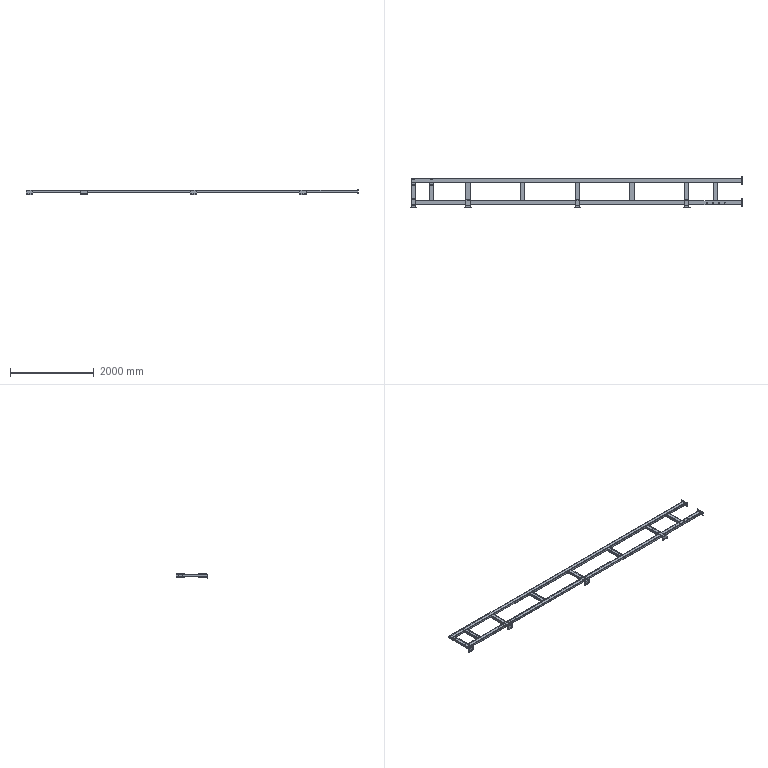Part | SolidWorks | features MirrorStock 1 | 22 solids | 386 faces | box 7924 x 758 x 126 mm | volume 27345410 mm3 | cylinder 194 | plane 192 | commonest cylinder face diameters 14 x64 8.4 x30 17 x30 20 x24 16 x16 12 x12